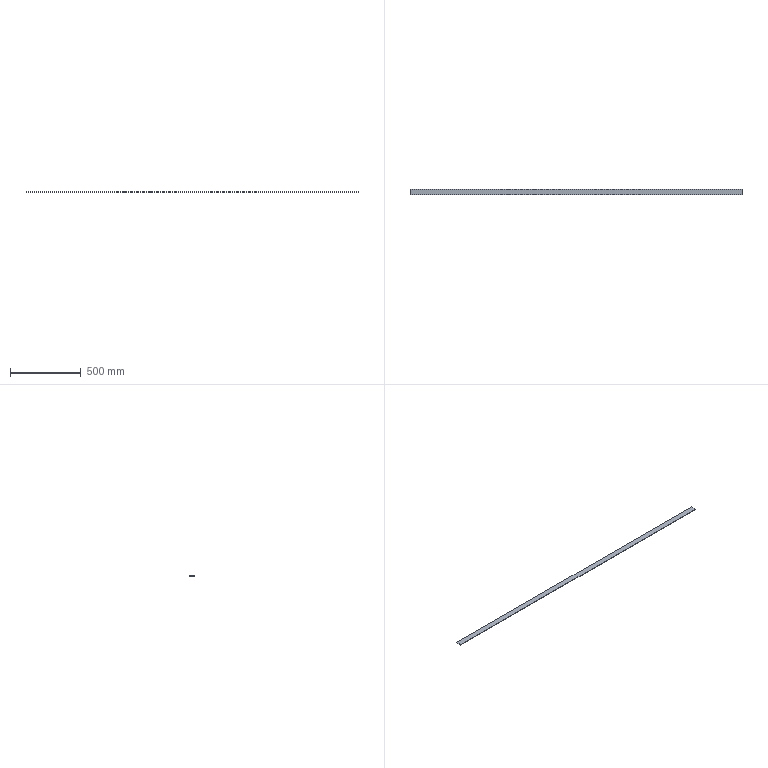Part | SolidWorks | features Extrusion 1 | 1 solid | 6 faces | box 2350 x 40 x 3 mm | volume 282000 mm3 | plane 6
STEP:
#1=CARTESIAN_POINT('',(0.,0.,0.));
#2=VERTEX_POINT('',#1);
#3=CARTESIAN_POINT('',(0.,-40.,0.));
#4=VERTEX_POINT('',#3);
#5=CARTESIAN_POINT('',(0.,0.,0.));
#6=DIRECTION('',(0.,-1.,0.));
#7=VECTOR('',#6,1000.);
#8=LINE('',#5,#7);
#9=EDGE_CURVE('',#2,#4,#8,.T.);
#10=ORIENTED_EDGE('',*,*,#9,.T.);
#11=CARTESIAN_POINT('',(0.,-40.,3.));
#12=VERTEX_POINT('',#11);
#13=CARTESIAN_POINT('',(0.,-40.,3.));
#14=DIRECTION('',(0.,0.,-1.));
#15=VECTOR('',#14,1000.);
#16=LINE('',#13,#15);
#17=EDGE_CURVE('',#12,#4,#16,.T.);
#18=ORIENTED_EDGE('',*,*,#17,.F.);
#19=CARTESIAN_POINT('',(0.,0.,3.));
#20=VERTEX_POINT('',#19);
#21=CARTESIAN_POINT('',(0.,0.,3.));
#22=DIRECTION('',(0.,-1.,0.));
#23=VECTOR('',#22,1000.);
#24=LINE('',#21,#23);
#25=EDGE_CURVE('',#20,#12,#24,.T.);
#26=ORIENTED_EDGE('',*,*,#25,.F.);
#27=CARTESIAN_POINT('',(0.,0.,3.));
#28=DIRECTION('',(0.,0.,-1.));
#29=VECTOR('',#28,1000.);
#30=LINE('',#27,#29);
#31=EDGE_CURVE('',#20,#2,#30,.T.);
#32=ORIENTED_EDGE('',*,*,#31,.T.);
#33=EDGE_LOOP('',(#10,#18,#26,#32));
#34=FACE_OUTER_BOUND('',#33,.T.);
#35=CARTESIAN_POINT('',(0.,0.,3.));
#36=DIRECTION('',(1.,0.,0.));
#37=DIRECTION('',(0.,1.,0.));
#38=AXIS2_PLACEMENT_3D('',#35,#36,#37);
#39=PLANE('',#38);
#40=ADVANCED_FACE('',(#34),#39,.F.);
#41=CARTESIAN_POINT('',(2350.,-40.,0.));
#42=VERTEX_POINT('',#41);
#43=CARTESIAN_POINT('',(0.,-40.,0.));
#44=DIRECTION('',(1.,0.,0.));
#45=VECTOR('',#44,1000.);
#46=LINE('',#43,#45);
#47=EDGE_CURVE('',#4,#42,#46,.T.);
#48=ORIENTED_EDGE('',*,*,#47,.T.);
#49=CARTESIAN_POINT('',(2350.,-40.,3.));
#50=VERTEX_POINT('',#49);
#51=CARTESIAN_POINT('',(2350.,-40.,3.));
#52=DIRECTION('',(0.,0.,-1.));
#53=VECTOR('',#52,1000.);
#54=LINE('',#51,#53);
#55=EDGE_CURVE('',#50,#42,#54,.T.);
#56=ORIENTED_EDGE('',*,*,#55,.F.);
#57=CARTESIAN_POINT('',(0.,-40.,3.));
#58=DIRECTION('',(1.,0.,0.));
#59=VECTOR('',#58,1000.);
#60=LINE('',#57,#59);
#61=EDGE_CURVE('',#12,#50,#60,.T.);
#62=ORIENTED_EDGE('',*,*,#61,.F.);
#63=ORIENTED_EDGE('',*,*,#17,.T.);
#64=EDGE_LOOP('',(#48,#56,#62,#63));
#65=FACE_OUTER_BOUND('',#64,.T.);
#66=CARTESIAN_POINT('',(0.,-40.,3.));
#67=DIRECTION('',(0.,1.,0.));
#68=DIRECTION('',(0.,0.,1.));
#69=AXIS2_PLACEMENT_3D('',#66,#67,#68);
#70=PLANE('',#69);
#71=ADVANCED_FACE('',(#65),#70,.F.);
#72=CARTESIAN_POINT('',(2350.,0.,0.));
#73=VERTEX_POINT('',#72);
#74=CARTESIAN_POINT('',(2350.,0.,0.));
#75=DIRECTION('',(0.,1.,0.));
#76=VECTOR('',#75,1000.);
#77=LINE('',#74,#76);
#78=EDGE_CURVE('',#42,#73,#77,.T.);
#79=ORIENTED_EDGE('',*,*,#78,.T.);
#80=CARTESIAN_POINT('',(2350.,0.,3.));
#81=VERTEX_POINT('',#80);
#82=CARTESIAN_POINT('',(2350.,0.,3.));
#83=DIRECTION('',(0.,0.,-1.));
#84=VECTOR('',#83,1000.);
#85=LINE('',#82,#84);
#86=EDGE_CURVE('',#81,#73,#85,.T.);
#87=ORIENTED_EDGE('',*,*,#86,.F.);
#88=CARTESIAN_POINT('',(2350.,0.,3.));
#89=DIRECTION('',(0.,1.,0.));
#90=VECTOR('',#89,1000.);
#91=LINE('',#88,#90);
#92=EDGE_CURVE('',#50,#81,#91,.T.);
#93=ORIENTED_EDGE('',*,*,#92,.F.);
#94=ORIENTED_EDGE('',*,*,#55,.T.);
#95=EDGE_LOOP('',(#79,#87,#93,#94));
#96=FACE_OUTER_BOUND('',#95,.T.);
#97=CARTESIAN_POINT('',(2350.,0.,3.));
#98=DIRECTION('',(-1.,0.,0.));
#99=DIRECTION('',(0.,0.,1.));
#100=AXIS2_PLACEMENT_3D('',#97,#98,#99);
#101=PLANE('',#100);
#102=ADVANCED_FACE('',(#96),#101,.F.);
#103=CARTESIAN_POINT('',(0.,0.,0.));
#104=DIRECTION('',(-1.,0.,0.));
#105=VECTOR('',#104,1000.);
#106=LINE('',#103,#105);
#107=EDGE_CURVE('',#73,#2,#106,.T.);
#108=ORIENTED_EDGE('',*,*,#107,.T.);
#109=ORIENTED_EDGE('',*,*,#31,.F.);
#110=CARTESIAN_POINT('',(0.,0.,3.));
#111=DIRECTION('',(-1.,0.,0.));
#112=VECTOR('',#111,1000.);
#113=LINE('',#110,#112);
#114=EDGE_CURVE('',#81,#20,#113,.T.);
#115=ORIENTED_EDGE('',*,*,#114,.F.);
#116=ORIENTED_EDGE('',*,*,#86,.T.);
#117=EDGE_LOOP('',(#108,#109,#115,#116));
#118=FACE_OUTER_BOUND('',#117,.T.);
#119=CARTESIAN_POINT('',(0.,0.,3.));
#120=DIRECTION('',(0.,-1.,0.));
#121=DIRECTION('',(0.,0.,-1.));
#122=AXIS2_PLACEMENT_3D('',#119,#120,#121);
#123=PLANE('',#122);
#124=ADVANCED_FACE('',(#118),#123,.F.);
#125=ORIENTED_EDGE('',*,*,#25,.T.);
#126=ORIENTED_EDGE('',*,*,#61,.T.);
#127=ORIENTED_EDGE('',*,*,#92,.T.);
#128=ORIENTED_EDGE('',*,*,#114,.T.);
#129=EDGE_LOOP('',(#125,#126,#127,#128));
#130=FACE_OUTER_BOUND('',#129,.T.);
#131=CARTESIAN_POINT('',(0.,0.,3.));
#132=DIRECTION('',(0.,0.,1.));
#133=DIRECTION('',(1.,0.,0.));
#134=AXIS2_PLACEMENT_3D('',#131,#132,#133);
#135=PLANE('',#134);
#136=ADVANCED_FACE('',(#130),#135,.T.);
#137=ORIENTED_EDGE('',*,*,#9,.F.);
#138=ORIENTED_EDGE('',*,*,#107,.F.);
#139=ORIENTED_EDGE('',*,*,#78,.F.);
#140=ORIENTED_EDGE('',*,*,#47,.F.);
#141=EDGE_LOOP('',(#137,#138,#139,#140));
#142=FACE_OUTER_BOUND('',#141,.T.);
#143=CARTESIAN_POINT('',(0.,0.,0.));
#144=DIRECTION('',(0.,0.,1.));
#145=DIRECTION('',(1.,0.,0.));
#146=AXIS2_PLACEMENT_3D('',#143,#144,#145);
#147=PLANE('',#146);
#148=ADVANCED_FACE('',(#142),#147,.F.);
#149=CLOSED_SHELL('',(#40,#71,#102,#124,#136,#148));
#150=MANIFOLD_SOLID_BREP('',#149);
#151=CARTESIAN_POINT('',(0.,0.,0.));
#152=DIRECTION('',(0.,0.,1.));
#153=DIRECTION('',(1.,0.,0.));
#154=AXIS2_PLACEMENT_3D('',#151,#152,#153);
#155=(LENGTH_UNIT()NAMED_UNIT(*)SI_UNIT(.MILLI.,.METRE.));
#156=UNCERTAINTY_MEASURE_WITH_UNIT(LENGTH_MEASURE(0.00001),#155,'','');
#157=(NAMED_UNIT(*)PLANE_ANGLE_UNIT()SI_UNIT($,.RADIAN.));
#158=(NAMED_UNIT(*)SI_UNIT($,.STERADIAN.)SOLID_ANGLE_UNIT());
#159=(GEOMETRIC_REPRESENTATION_CONTEXT(3)GLOBAL_UNCERTAINTY_ASSIGNED_CONTEXT((#156))GLOBAL_UNIT_ASSIGNED_CONTEXT((#155,#157,#158))REPRESENTATION_CONTEXT('',''));
#160=ADVANCED_BREP_SHAPE_REPRESENTATION('',(#150,#154),#159);